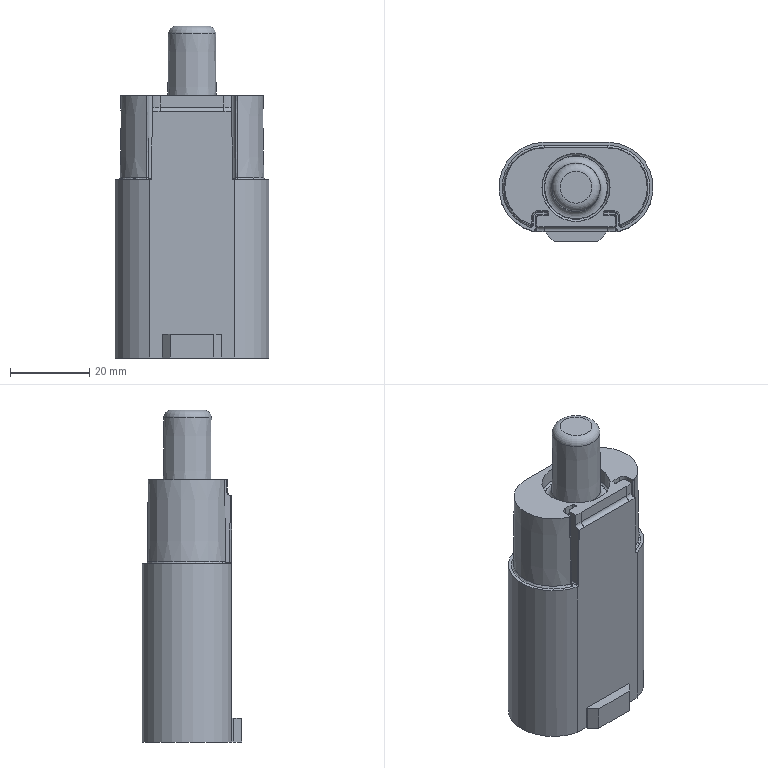Part | STEP file | lll_id230_x_t | 1 solid | 78 faces | box 38.894 x 25.019 x 83.75 mm | volume 50062 mm3 | plane 25 | cylinder 22 | spline 18 | torus 7 | cone 6 | commonest cylinder face diameters 0.602 x12 1.004 x3 2.008 x2 3.012 x2 22.83 x2 2.247 x1